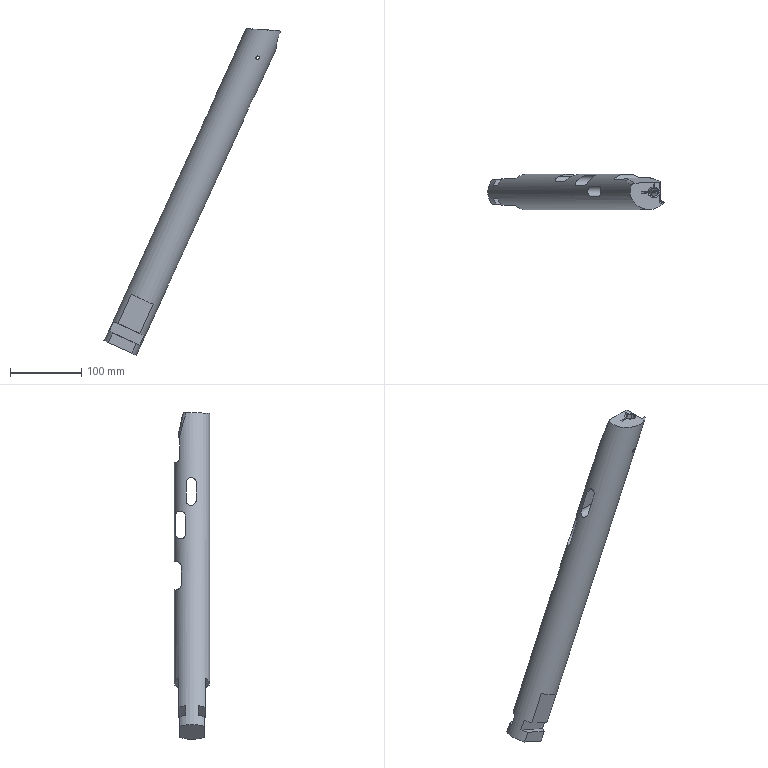Part | STEP file | solid 96 | 1 solid | 161 faces | box 247.177 x 50 x 457.681 mm | volume 845709 mm3 | plane 68 | other 59 | cylinder 15 | spline 14 | cone 3 | torus 2 | commonest cylinder face diameters 14 x8 5 x2 6 x2 4.02 x1 10 x1 50 x1